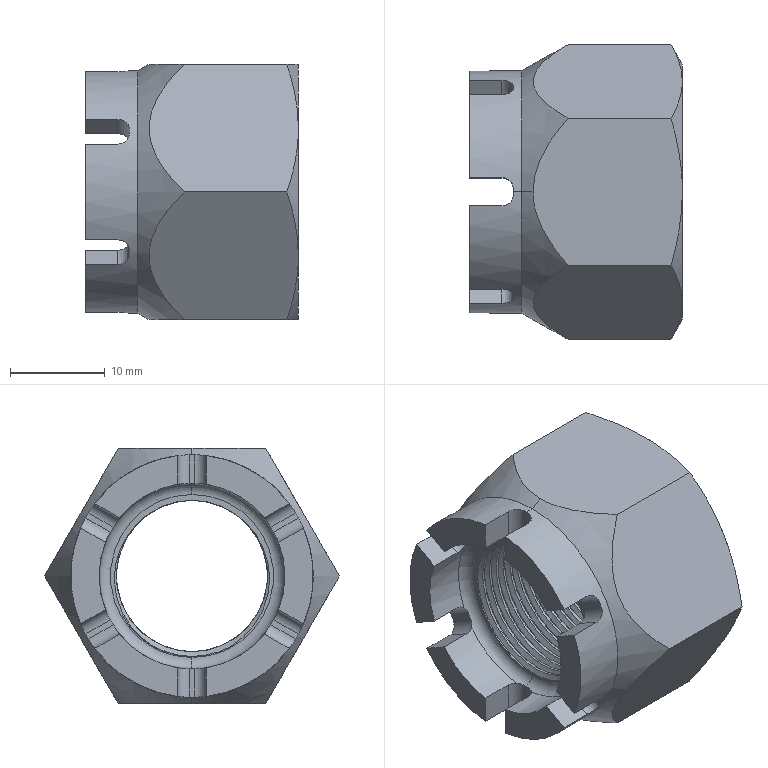Part | STEP file | Completa.sldasm-Part-61_Valor predeterminado | 1 solid | 136 faces | box 22.5 x 31.177 x 27 mm | volume 7880 mm3 | cylinder 92 | plane 32 | cone 8 | torus 2 | spline 2 | commonest cylinder face diameters 16 x36 17 x36 2.4 x12 19.65 x6 25.65 x2